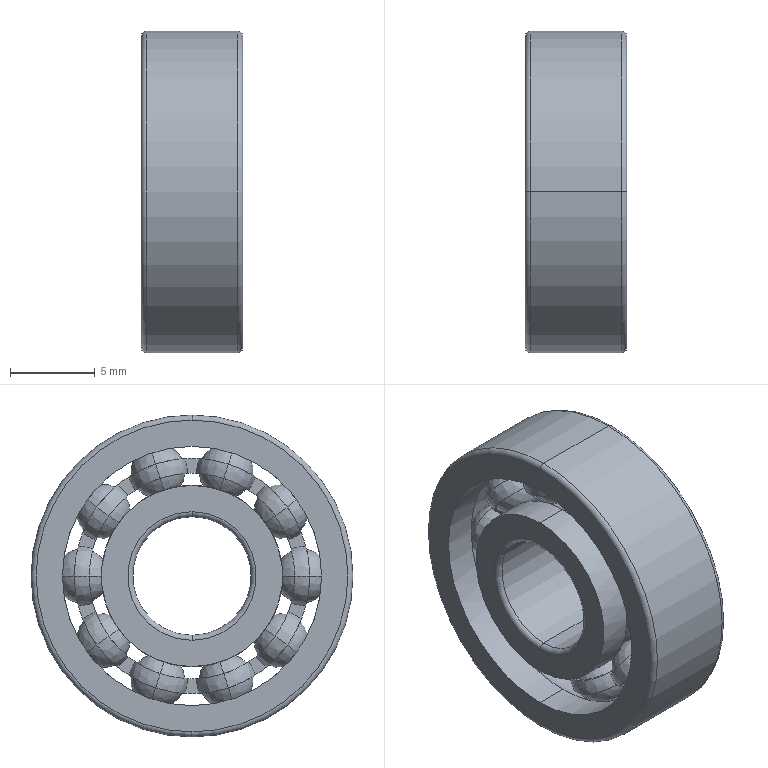Part | NX | features BREP 1 | 1 solid | 161 faces | box 6 x 19 x 19 mm | volume 1040 mm3 | sphere 80 | torus 41 | plane 24 | cylinder 16 | commonest cylinder face diameters 10.7 x4 15.3 x4 7 x2 12.12 x2 13.88 x2 19 x2